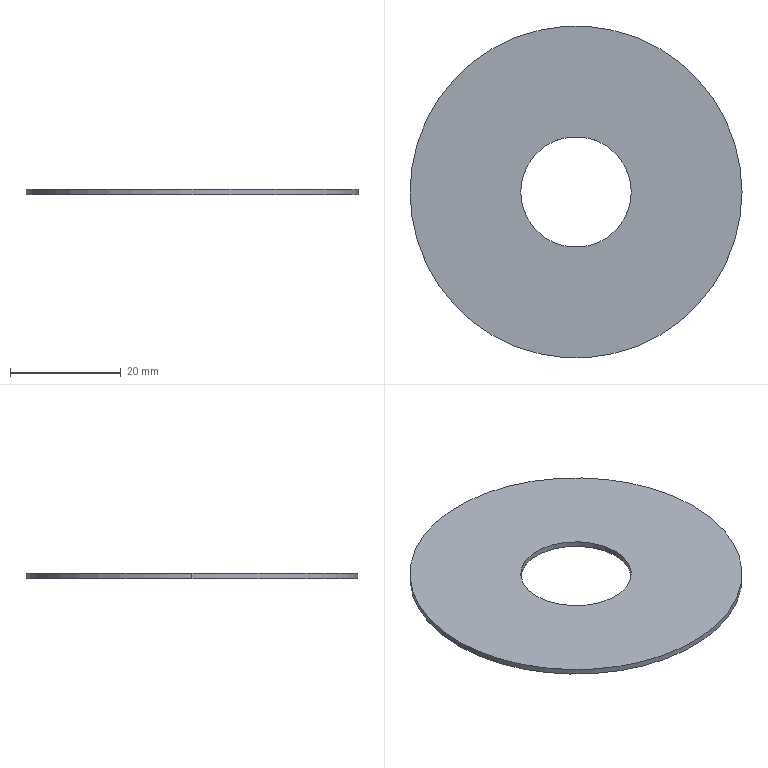Part | SolidWorks | features Extrusion 1 | 1 solid | 6 faces | box 60 x 60 x 1 mm | volume 2513 mm3 | cylinder 4 | plane 2 | commonest cylinder face diameters 20 x2 60 x2
STEP:
#1=CARTESIAN_POINT('',(-10.,0.,0.5));
#2=VERTEX_POINT('',#1);
#3=CARTESIAN_POINT('',(10.,0.,0.5));
#4=VERTEX_POINT('',#3);
#5=CARTESIAN_POINT('',(0.,0.,0.5));
#6=DIRECTION('',(0.,0.,1.));
#7=DIRECTION('',(1.,0.,0.));
#8=AXIS2_PLACEMENT_3D('',#5,#6,#7);
#9=CIRCLE('',#8,10.);
#10=EDGE_CURVE('',#2,#4,#9,.T.);
#11=ORIENTED_EDGE('',*,*,#10,.T.);
#12=CARTESIAN_POINT('',(10.,0.,-0.5));
#13=VERTEX_POINT('',#12);
#14=CARTESIAN_POINT('',(10.,0.,0.5));
#15=DIRECTION('',(0.,0.,-1.));
#16=VECTOR('',#15,1000.);
#17=LINE('',#14,#16);
#18=EDGE_CURVE('',#4,#13,#17,.T.);
#19=ORIENTED_EDGE('',*,*,#18,.T.);
#20=CARTESIAN_POINT('',(-10.,0.,-0.5));
#21=VERTEX_POINT('',#20);
#22=CARTESIAN_POINT('',(0.,0.,-0.5));
#23=DIRECTION('',(0.,0.,1.));
#24=DIRECTION('',(1.,0.,0.));
#25=AXIS2_PLACEMENT_3D('',#22,#23,#24);
#26=CIRCLE('',#25,10.);
#27=EDGE_CURVE('',#21,#13,#26,.T.);
#28=ORIENTED_EDGE('',*,*,#27,.F.);
#29=CARTESIAN_POINT('',(-10.,0.,0.5));
#30=DIRECTION('',(0.,0.,-1.));
#31=VECTOR('',#30,1000.);
#32=LINE('',#29,#31);
#33=EDGE_CURVE('',#2,#21,#32,.T.);
#34=ORIENTED_EDGE('',*,*,#33,.F.);
#35=EDGE_LOOP('',(#11,#19,#28,#34));
#36=FACE_OUTER_BOUND('',#35,.T.);
#37=CARTESIAN_POINT('',(0.,0.,0.5));
#38=DIRECTION('',(0.,0.,-1.));
#39=DIRECTION('',(-1.,0.,0.));
#40=AXIS2_PLACEMENT_3D('',#37,#38,#39);
#41=CYLINDRICAL_SURFACE('',#40,10.);
#42=ADVANCED_FACE('',(#36),#41,.F.);
#43=CARTESIAN_POINT('',(30.,0.,0.5));
#44=VERTEX_POINT('',#43);
#45=CARTESIAN_POINT('',(-30.,0.,0.5));
#46=VERTEX_POINT('',#45);
#47=CARTESIAN_POINT('',(0.,0.,0.5));
#48=DIRECTION('',(0.,0.,1.));
#49=DIRECTION('',(1.,0.,0.));
#50=AXIS2_PLACEMENT_3D('',#47,#48,#49);
#51=CIRCLE('',#50,30.);
#52=EDGE_CURVE('',#44,#46,#51,.T.);
#53=ORIENTED_EDGE('',*,*,#52,.F.);
#54=CARTESIAN_POINT('',(30.,0.,-0.5));
#55=VERTEX_POINT('',#54);
#56=CARTESIAN_POINT('',(30.,0.,0.5));
#57=DIRECTION('',(0.,0.,-1.));
#58=VECTOR('',#57,1000.);
#59=LINE('',#56,#58);
#60=EDGE_CURVE('',#44,#55,#59,.T.);
#61=ORIENTED_EDGE('',*,*,#60,.T.);
#62=CARTESIAN_POINT('',(-30.,0.,-0.5));
#63=VERTEX_POINT('',#62);
#64=CARTESIAN_POINT('',(0.,0.,-0.5));
#65=DIRECTION('',(0.,0.,1.));
#66=DIRECTION('',(1.,0.,0.));
#67=AXIS2_PLACEMENT_3D('',#64,#65,#66);
#68=CIRCLE('',#67,30.);
#69=EDGE_CURVE('',#55,#63,#68,.T.);
#70=ORIENTED_EDGE('',*,*,#69,.T.);
#71=CARTESIAN_POINT('',(-30.,0.,0.5));
#72=DIRECTION('',(0.,0.,-1.));
#73=VECTOR('',#72,1000.);
#74=LINE('',#71,#73);
#75=EDGE_CURVE('',#46,#63,#74,.T.);
#76=ORIENTED_EDGE('',*,*,#75,.F.);
#77=EDGE_LOOP('',(#53,#61,#70,#76));
#78=FACE_OUTER_BOUND('',#77,.T.);
#79=CARTESIAN_POINT('',(0.,0.,0.5));
#80=DIRECTION('',(0.,0.,-1.));
#81=DIRECTION('',(-1.,0.,0.));
#82=AXIS2_PLACEMENT_3D('',#79,#80,#81);
#83=CYLINDRICAL_SURFACE('',#82,30.);
#84=ADVANCED_FACE('',(#78),#83,.T.);
#85=CARTESIAN_POINT('',(0.,0.,0.5));
#86=DIRECTION('',(0.,0.,1.));
#87=DIRECTION('',(1.,0.,0.));
#88=AXIS2_PLACEMENT_3D('',#85,#86,#87);
#89=CIRCLE('',#88,30.);
#90=EDGE_CURVE('',#46,#44,#89,.T.);
#91=ORIENTED_EDGE('',*,*,#90,.T.);
#92=ORIENTED_EDGE('',*,*,#52,.T.);
#93=EDGE_LOOP('',(#91,#92));
#94=FACE_OUTER_BOUND('',#93,.T.);
#95=ORIENTED_EDGE('',*,*,#10,.F.);
#96=CARTESIAN_POINT('',(0.,0.,0.5));
#97=DIRECTION('',(0.,0.,1.));
#98=DIRECTION('',(1.,0.,0.));
#99=AXIS2_PLACEMENT_3D('',#96,#97,#98);
#100=CIRCLE('',#99,10.);
#101=EDGE_CURVE('',#4,#2,#100,.T.);
#102=ORIENTED_EDGE('',*,*,#101,.F.);
#103=EDGE_LOOP('',(#95,#102));
#104=FACE_BOUND('',#103,.T.);
#105=CARTESIAN_POINT('',(0.,0.,0.5));
#106=DIRECTION('',(0.,0.,1.));
#107=DIRECTION('',(1.,0.,0.));
#108=AXIS2_PLACEMENT_3D('',#105,#106,#107);
#109=PLANE('',#108);
#110=ADVANCED_FACE('',(#94,#104),#109,.T.);
#111=CARTESIAN_POINT('',(0.,0.,-0.5));
#112=DIRECTION('',(0.,0.,1.));
#113=DIRECTION('',(1.,0.,0.));
#114=AXIS2_PLACEMENT_3D('',#111,#112,#113);
#115=CIRCLE('',#114,30.);
#116=EDGE_CURVE('',#63,#55,#115,.T.);
#117=ORIENTED_EDGE('',*,*,#116,.F.);
#118=ORIENTED_EDGE('',*,*,#69,.F.);
#119=EDGE_LOOP('',(#117,#118));
#120=FACE_OUTER_BOUND('',#119,.T.);
#121=ORIENTED_EDGE('',*,*,#27,.T.);
#122=CARTESIAN_POINT('',(0.,0.,-0.5));
#123=DIRECTION('',(0.,0.,1.));
#124=DIRECTION('',(1.,0.,0.));
#125=AXIS2_PLACEMENT_3D('',#122,#123,#124);
#126=CIRCLE('',#125,10.);
#127=EDGE_CURVE('',#13,#21,#126,.T.);
#128=ORIENTED_EDGE('',*,*,#127,.T.);
#129=EDGE_LOOP('',(#121,#128));
#130=FACE_BOUND('',#129,.T.);
#131=CARTESIAN_POINT('',(0.,0.,-0.5));
#132=DIRECTION('',(0.,0.,1.));
#133=DIRECTION('',(1.,0.,0.));
#134=AXIS2_PLACEMENT_3D('',#131,#132,#133);
#135=PLANE('',#134);
#136=ADVANCED_FACE('',(#120,#130),#135,.F.);
#137=ORIENTED_EDGE('',*,*,#60,.F.);
#138=ORIENTED_EDGE('',*,*,#90,.F.);
#139=ORIENTED_EDGE('',*,*,#75,.T.);
#140=ORIENTED_EDGE('',*,*,#116,.T.);
#141=EDGE_LOOP('',(#137,#138,#139,#140));
#142=FACE_OUTER_BOUND('',#141,.T.);
#143=CARTESIAN_POINT('',(0.,0.,0.5));
#144=DIRECTION('',(0.,0.,-1.));
#145=DIRECTION('',(-1.,0.,0.));
#146=AXIS2_PLACEMENT_3D('',#143,#144,#145);
#147=CYLINDRICAL_SURFACE('',#146,30.);
#148=ADVANCED_FACE('',(#142),#147,.T.);
#149=ORIENTED_EDGE('',*,*,#18,.F.);
#150=ORIENTED_EDGE('',*,*,#101,.T.);
#151=ORIENTED_EDGE('',*,*,#33,.T.);
#152=ORIENTED_EDGE('',*,*,#127,.F.);
#153=EDGE_LOOP('',(#149,#150,#151,#152));
#154=FACE_OUTER_BOUND('',#153,.T.);
#155=CARTESIAN_POINT('',(0.,0.,0.5));
#156=DIRECTION('',(0.,0.,-1.));
#157=DIRECTION('',(-1.,0.,0.));
#158=AXIS2_PLACEMENT_3D('',#155,#156,#157);
#159=CYLINDRICAL_SURFACE('',#158,10.);
#160=ADVANCED_FACE('',(#154),#159,.F.);
#161=CLOSED_SHELL('',(#42,#84,#110,#136,#148,#160));
#162=MANIFOLD_SOLID_BREP('',#161);
#163=CARTESIAN_POINT('',(0.,0.,0.));
#164=DIRECTION('',(0.,0.,1.));
#165=DIRECTION('',(1.,0.,0.));
#166=AXIS2_PLACEMENT_3D('',#163,#164,#165);
#167=(LENGTH_UNIT()NAMED_UNIT(*)SI_UNIT(.MILLI.,.METRE.));
#168=UNCERTAINTY_MEASURE_WITH_UNIT(LENGTH_MEASURE(0.00001),#167,'','');
#169=(NAMED_UNIT(*)PLANE_ANGLE_UNIT()SI_UNIT($,.RADIAN.));
#170=(NAMED_UNIT(*)SI_UNIT($,.STERADIAN.)SOLID_ANGLE_UNIT());
#171=(GEOMETRIC_REPRESENTATION_CONTEXT(3)GLOBAL_UNCERTAINTY_ASSIGNED_CONTEXT((#168))GLOBAL_UNIT_ASSIGNED_CONTEXT((#167,#169,#170))REPRESENTATION_CONTEXT('',''));
#172=ADVANCED_BREP_SHAPE_REPRESENTATION('',(#162,#166),#171);